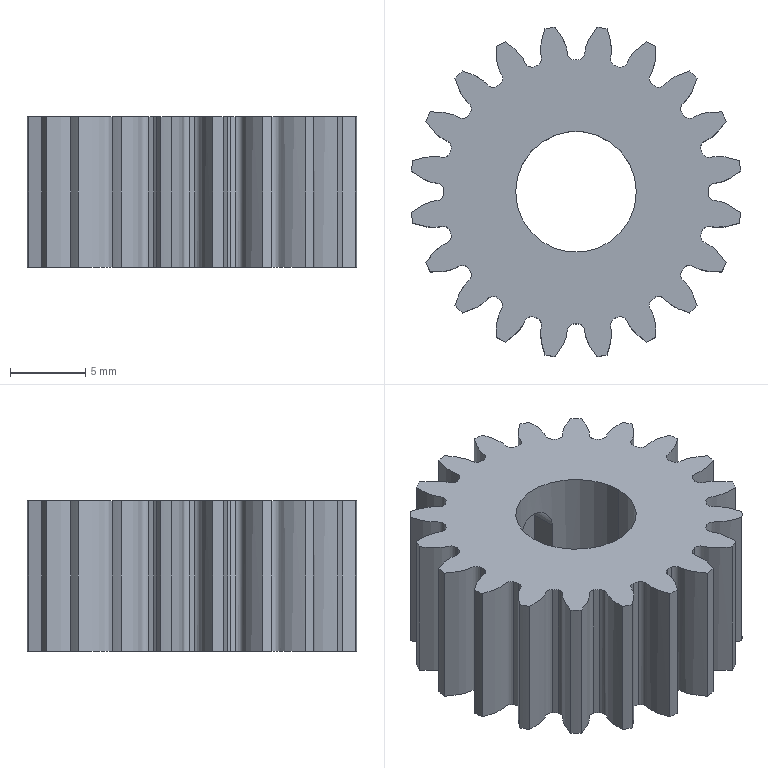Part | SolidWorks | features ICE 3, CirPattern 1, Extrusion 1, RefAxis 1 | 1 solid | 88 faces | box 21.827 x 21.827 x 10 mm | volume 2548 mm3 | cylinder 43 | spline 40 | plane 5 | commonest cylinder face diameters 17.5 x20 22 x20 8 x2 3 x1